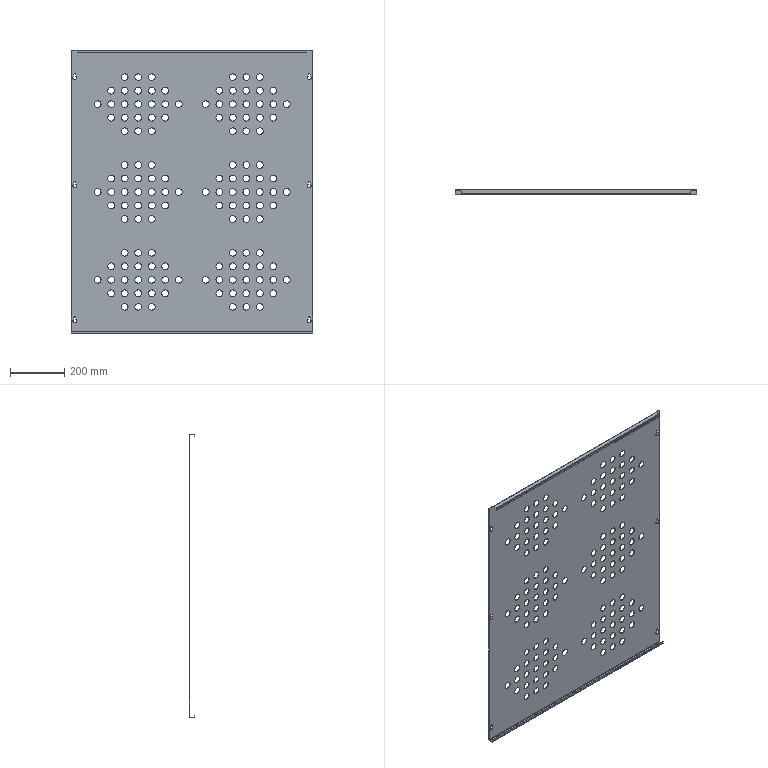Part | NX | features solid 2 | 1 solid | 342 faces | box 892 x 20 x 1050 mm | volume 1366900 mm3 | cylinder 308 | plane 34 | commonest cylinder face diameters 25 x276 14 x18 7 x6 3 x4 6 x4